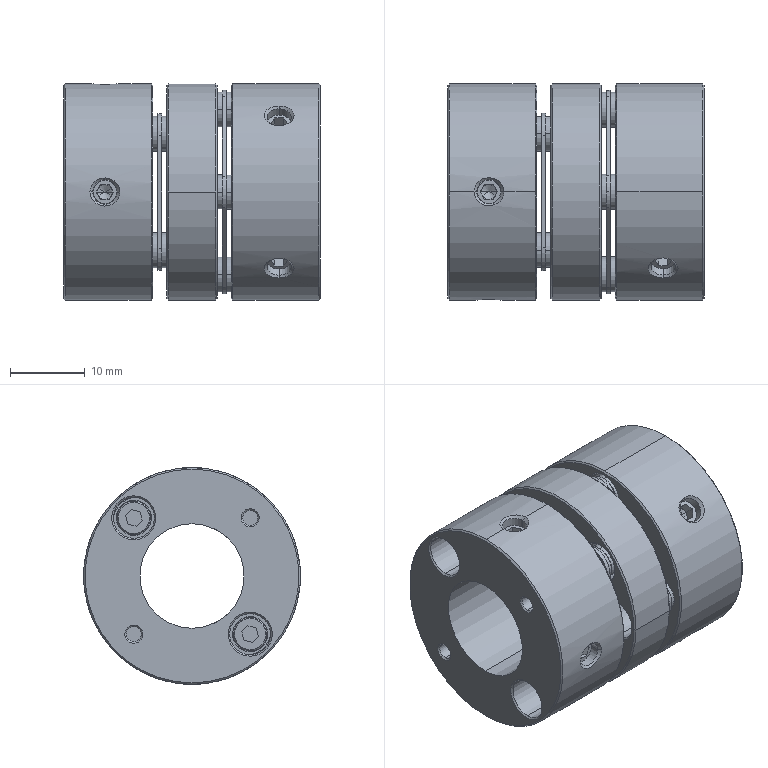Part | SolidWorks | features BaseBody 5 | 5 solids | 403 faces | box 34.3 x 29 x 29 mm | volume 14180 mm3 | plane 154 | cone 128 | cylinder 121 | commonest cylinder face diameters 4.7 x32 2.013 x16 4.5 x16 5.5 x16 6 x9 3.242 x8